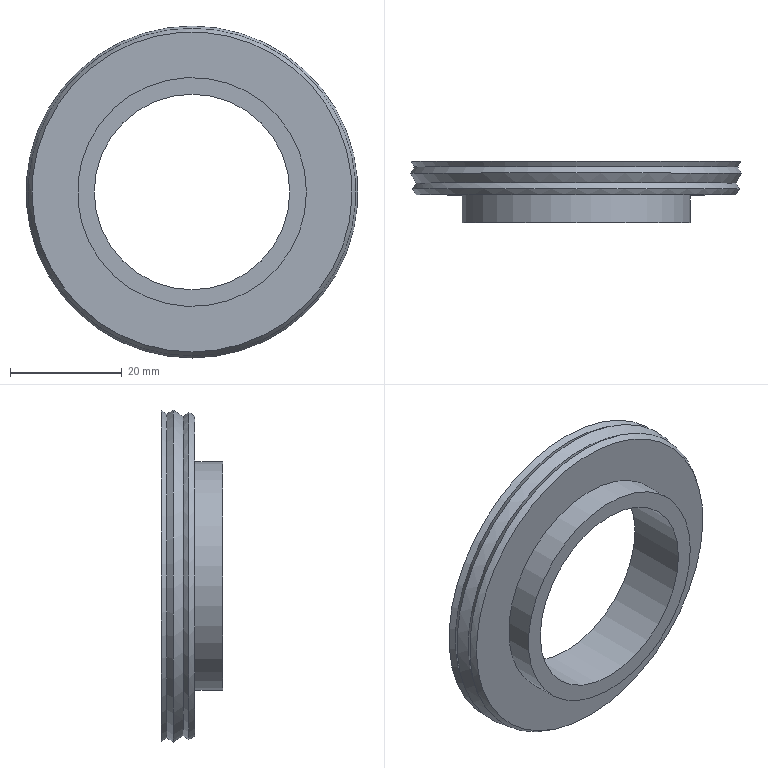Part | NX | features DATUM_CSYS 5, SKETCH 4, EXTRUDE 3, SWP104 1 | 1 solid | 10 faces | box 59.468 x 11 x 59.468 mm | volume 12056 mm3 | cone 5 | plane 3 | cylinder 2 | commonest cylinder face diameters 35 x1 41 x1
STEP:
#1=CARTESIAN_POINT('',(20.5,-6.,0.));
#2=VERTEX_POINT('',#1);
#3=CARTESIAN_POINT('',(0.,-6.,0.));
#4=DIRECTION('',(0.,-1.,0.));
#5=DIRECTION('',(1.,0.,0.));
#6=AXIS2_PLACEMENT_3D('',#3,#4,#5);
#7=CIRCLE('',#6,20.5);
#8=EDGE_CURVE('',#2,#2,#7,.T.);
#9=ORIENTED_EDGE('',*,*,#8,.F.);
#10=EDGE_LOOP('',(#9));
#11=FACE_BOUND('',#10,.T.);
#12=CARTESIAN_POINT('',(0.,-6.,-28.661));
#13=VERTEX_POINT('',#12);
#14=CARTESIAN_POINT('',(0.,-6.,0.));
#15=DIRECTION('',(0.,-1.,0.));
#16=DIRECTION('',(0.,0.,-1.));
#17=AXIS2_PLACEMENT_3D('',#14,#15,#16);
#18=CIRCLE('',#17,28.661);
#19=EDGE_CURVE('',#13,#13,#18,.T.);
#20=ORIENTED_EDGE('',*,*,#19,.T.);
#21=EDGE_LOOP('',(#20));
#22=FACE_BOUND('',#21,.T.);
#23=CARTESIAN_POINT('',(0.,-6.,0.));
#24=DIRECTION('',(0.,-1.,0.));
#25=DIRECTION('',(0.,0.,-1.));
#26=AXIS2_PLACEMENT_3D('',#23,#24,#25);
#27=PLANE('',#26);
#28=ADVANCED_FACE('',(#11,#22),#27,.T.);
#29=CARTESIAN_POINT('',(20.5,-11.,0.));
#30=VERTEX_POINT('',#29);
#31=CARTESIAN_POINT('',(0.,-11.,0.));
#32=DIRECTION('',(0.,-1.,0.));
#33=DIRECTION('',(1.,0.,0.));
#34=AXIS2_PLACEMENT_3D('',#31,#32,#33);
#35=CIRCLE('',#34,20.5);
#36=EDGE_CURVE('',#30,#30,#35,.T.);
#37=ORIENTED_EDGE('',*,*,#36,.F.);
#38=EDGE_LOOP('',(#37));
#39=FACE_BOUND('',#38,.T.);
#40=ORIENTED_EDGE('',*,*,#8,.T.);
#41=EDGE_LOOP('',(#40));
#42=FACE_BOUND('',#41,.T.);
#43=CARTESIAN_POINT('',(0.,-11.,0.));
#44=DIRECTION('',(0.,1.,0.));
#45=DIRECTION('',(0.,0.,1.));
#46=AXIS2_PLACEMENT_3D('',#43,#44,#45);
#47=CYLINDRICAL_SURFACE('',#46,20.5);
#48=ADVANCED_FACE('',(#39,#42),#47,.T.);
#49=CARTESIAN_POINT('',(0.,-11.,-17.5));
#50=VERTEX_POINT('',#49);
#51=CARTESIAN_POINT('',(0.,-11.,0.));
#52=DIRECTION('',(0.,-1.,0.));
#53=DIRECTION('',(0.,0.,-1.));
#54=AXIS2_PLACEMENT_3D('',#51,#52,#53);
#55=CIRCLE('',#54,17.5);
#56=EDGE_CURVE('',#50,#50,#55,.F.);
#57=ORIENTED_EDGE('',*,*,#56,.T.);
#58=EDGE_LOOP('',(#57));
#59=FACE_BOUND('',#58,.T.);
#60=ORIENTED_EDGE('',*,*,#36,.T.);
#61=EDGE_LOOP('',(#60));
#62=FACE_BOUND('',#61,.T.);
#63=CARTESIAN_POINT('',(0.,-11.,0.));
#64=DIRECTION('',(0.,-1.,0.));
#65=DIRECTION('',(0.,0.,-1.));
#66=AXIS2_PLACEMENT_3D('',#63,#64,#65);
#67=PLANE('',#66);
#68=ADVANCED_FACE('',(#59,#62),#67,.T.);
#69=CARTESIAN_POINT('',(0.,-1.,-29.));
#70=VERTEX_POINT('',#69);
#71=CARTESIAN_POINT('',(0.,-1.,0.));
#72=DIRECTION('',(0.,-1.,0.));
#73=DIRECTION('',(0.,0.,-1.));
#74=AXIS2_PLACEMENT_3D('',#71,#72,#73);
#75=CIRCLE('',#74,29.);
#76=EDGE_CURVE('',#70,#70,#75,.F.);
#77=ORIENTED_EDGE('',*,*,#76,.T.);
#78=EDGE_LOOP('',(#77));
#79=FACE_BOUND('',#78,.T.);
#80=CARTESIAN_POINT('',(0.,0.,-29.623));
#81=VERTEX_POINT('',#80);
#82=CARTESIAN_POINT('',(0.,0.,0.));
#83=DIRECTION('',(0.,-1.,0.));
#84=DIRECTION('',(0.,0.,-1.));
#85=AXIS2_PLACEMENT_3D('',#82,#83,#84);
#86=CIRCLE('',#85,29.623);
#87=EDGE_CURVE('',#81,#81,#86,.T.);
#88=ORIENTED_EDGE('',*,*,#87,.T.);
#89=EDGE_LOOP('',(#88));
#90=FACE_BOUND('',#89,.T.);
#91=CARTESIAN_POINT('',(0.,-1.,0.));
#92=DIRECTION('',(0.,1.,0.));
#93=DIRECTION('',(0.,0.,1.));
#94=AXIS2_PLACEMENT_3D('',#91,#92,#93);
#95=CONICAL_SURFACE('',#94,29.,0.5574);
#96=ADVANCED_FACE('',(#79,#90),#95,.T.);
#97=ORIENTED_EDGE('',*,*,#19,.F.);
#98=EDGE_LOOP('',(#97));
#99=FACE_BOUND('',#98,.T.);
#100=CARTESIAN_POINT('',(0.,-4.953,-29.314));
#101=VERTEX_POINT('',#100);
#102=CARTESIAN_POINT('',(0.,-4.953,0.));
#103=DIRECTION('',(0.,-1.,0.));
#104=DIRECTION('',(0.,0.,-1.));
#105=AXIS2_PLACEMENT_3D('',#102,#103,#104);
#106=CIRCLE('',#105,29.314);
#107=EDGE_CURVE('',#101,#101,#106,.F.);
#108=ORIENTED_EDGE('',*,*,#107,.F.);
#109=EDGE_LOOP('',(#108));
#110=FACE_BOUND('',#109,.T.);
#111=CARTESIAN_POINT('',(0.,-6.121,0.));
#112=DIRECTION('',(0.,1.,0.));
#113=DIRECTION('',(0.,0.,1.));
#114=AXIS2_PLACEMENT_3D('',#111,#112,#113);
#115=CONICAL_SURFACE('',#114,28.586,0.5574);
#116=ADVANCED_FACE('',(#99,#110),#115,.T.);
#117=CARTESIAN_POINT('',(0.,-3.9,-28.631));
#118=VERTEX_POINT('',#117);
#119=CARTESIAN_POINT('',(0.,-3.9,0.));
#120=DIRECTION('',(0.,-1.,0.));
#121=DIRECTION('',(0.,0.,-1.));
#122=AXIS2_PLACEMENT_3D('',#119,#120,#121);
#123=CIRCLE('',#122,28.631);
#124=EDGE_CURVE('',#118,#118,#123,.F.);
#125=ORIENTED_EDGE('',*,*,#124,.F.);
#126=EDGE_LOOP('',(#125));
#127=FACE_BOUND('',#126,.T.);
#128=ORIENTED_EDGE('',*,*,#107,.T.);
#129=EDGE_LOOP('',(#128));
#130=FACE_BOUND('',#129,.T.);
#131=CARTESIAN_POINT('',(0.,-4.953,0.));
#132=DIRECTION('',(0.,-1.,0.));
#133=DIRECTION('',(0.,0.,-1.));
#134=AXIS2_PLACEMENT_3D('',#131,#132,#133);
#135=CONICAL_SURFACE('',#134,29.314,0.5756);
#136=ADVANCED_FACE('',(#127,#130),#135,.T.);
#137=CARTESIAN_POINT('',(0.,-2.131,-29.734));
#138=VERTEX_POINT('',#137);
#139=CARTESIAN_POINT('',(0.,-2.131,0.));
#140=DIRECTION('',(0.,-1.,0.));
#141=DIRECTION('',(0.,0.,-1.));
#142=AXIS2_PLACEMENT_3D('',#139,#140,#141);
#143=CIRCLE('',#142,29.734);
#144=EDGE_CURVE('',#138,#138,#143,.F.);
#145=ORIENTED_EDGE('',*,*,#144,.F.);
#146=EDGE_LOOP('',(#145));
#147=FACE_BOUND('',#146,.T.);
#148=ORIENTED_EDGE('',*,*,#124,.T.);
#149=EDGE_LOOP('',(#148));
#150=FACE_BOUND('',#149,.T.);
#151=CARTESIAN_POINT('',(0.,-3.9,0.));
#152=DIRECTION('',(0.,1.,0.));
#153=DIRECTION('',(0.,0.,1.));
#154=AXIS2_PLACEMENT_3D('',#151,#152,#153);
#155=CONICAL_SURFACE('',#154,28.631,0.5574);
#156=ADVANCED_FACE('',(#147,#150),#155,.T.);
#157=ORIENTED_EDGE('',*,*,#76,.F.);
#158=EDGE_LOOP('',(#157));
#159=FACE_BOUND('',#158,.T.);
#160=ORIENTED_EDGE('',*,*,#144,.T.);
#161=EDGE_LOOP('',(#160));
#162=FACE_BOUND('',#161,.T.);
#163=CARTESIAN_POINT('',(0.,-2.131,0.));
#164=DIRECTION('',(0.,-1.,0.));
#165=DIRECTION('',(0.,0.,-1.));
#166=AXIS2_PLACEMENT_3D('',#163,#164,#165);
#167=CONICAL_SURFACE('',#166,29.734,0.5756);
#168=ADVANCED_FACE('',(#159,#162),#167,.T.);
#169=CARTESIAN_POINT('',(0.,0.,-17.5));
#170=VERTEX_POINT('',#169);
#171=CARTESIAN_POINT('',(0.,0.,0.));
#172=DIRECTION('',(0.,-1.,0.));
#173=DIRECTION('',(0.,0.,-1.));
#174=AXIS2_PLACEMENT_3D('',#171,#172,#173);
#175=CIRCLE('',#174,17.5);
#176=EDGE_CURVE('',#170,#170,#175,.F.);
#177=ORIENTED_EDGE('',*,*,#176,.F.);
#178=EDGE_LOOP('',(#177));
#179=FACE_BOUND('',#178,.T.);
#180=ORIENTED_EDGE('',*,*,#87,.F.);
#181=EDGE_LOOP('',(#180));
#182=FACE_BOUND('',#181,.T.);
#183=CARTESIAN_POINT('',(0.,0.,0.));
#184=DIRECTION('',(0.,-1.,0.));
#185=DIRECTION('',(0.,0.,-1.));
#186=AXIS2_PLACEMENT_3D('',#183,#184,#185);
#187=PLANE('',#186);
#188=ADVANCED_FACE('',(#179,#182),#187,.F.);
#189=ORIENTED_EDGE('',*,*,#56,.F.);
#190=EDGE_LOOP('',(#189));
#191=FACE_BOUND('',#190,.T.);
#192=ORIENTED_EDGE('',*,*,#176,.T.);
#193=EDGE_LOOP('',(#192));
#194=FACE_BOUND('',#193,.T.);
#195=CARTESIAN_POINT('',(0.,-28.,0.));
#196=DIRECTION('',(0.,1.,0.));
#197=DIRECTION('',(0.,0.,1.));
#198=AXIS2_PLACEMENT_3D('',#195,#196,#197);
#199=CYLINDRICAL_SURFACE('',#198,17.5);
#200=ADVANCED_FACE('',(#191,#194),#199,.F.);
#201=CLOSED_SHELL('',(#28,#48,#68,#96,#116,#136,#156,#168,#188,#200));
#202=MANIFOLD_SOLID_BREP('',#201);
#203=(LENGTH_UNIT()NAMED_UNIT(*)SI_UNIT(.MILLI.,.METRE.));
#204=UNCERTAINTY_MEASURE_WITH_UNIT(LENGTH_MEASURE(0.00001),#203,'','');
#205=(NAMED_UNIT(*)PLANE_ANGLE_UNIT()SI_UNIT($,.RADIAN.));
#206=(NAMED_UNIT(*)SI_UNIT($,.STERADIAN.)SOLID_ANGLE_UNIT());
#207=(GEOMETRIC_REPRESENTATION_CONTEXT(3)GLOBAL_UNCERTAINTY_ASSIGNED_CONTEXT((#204))GLOBAL_UNIT_ASSIGNED_CONTEXT((#203,#205,#206))REPRESENTATION_CONTEXT('',''));
#208=ADVANCED_BREP_SHAPE_REPRESENTATION('',(#202),#207);